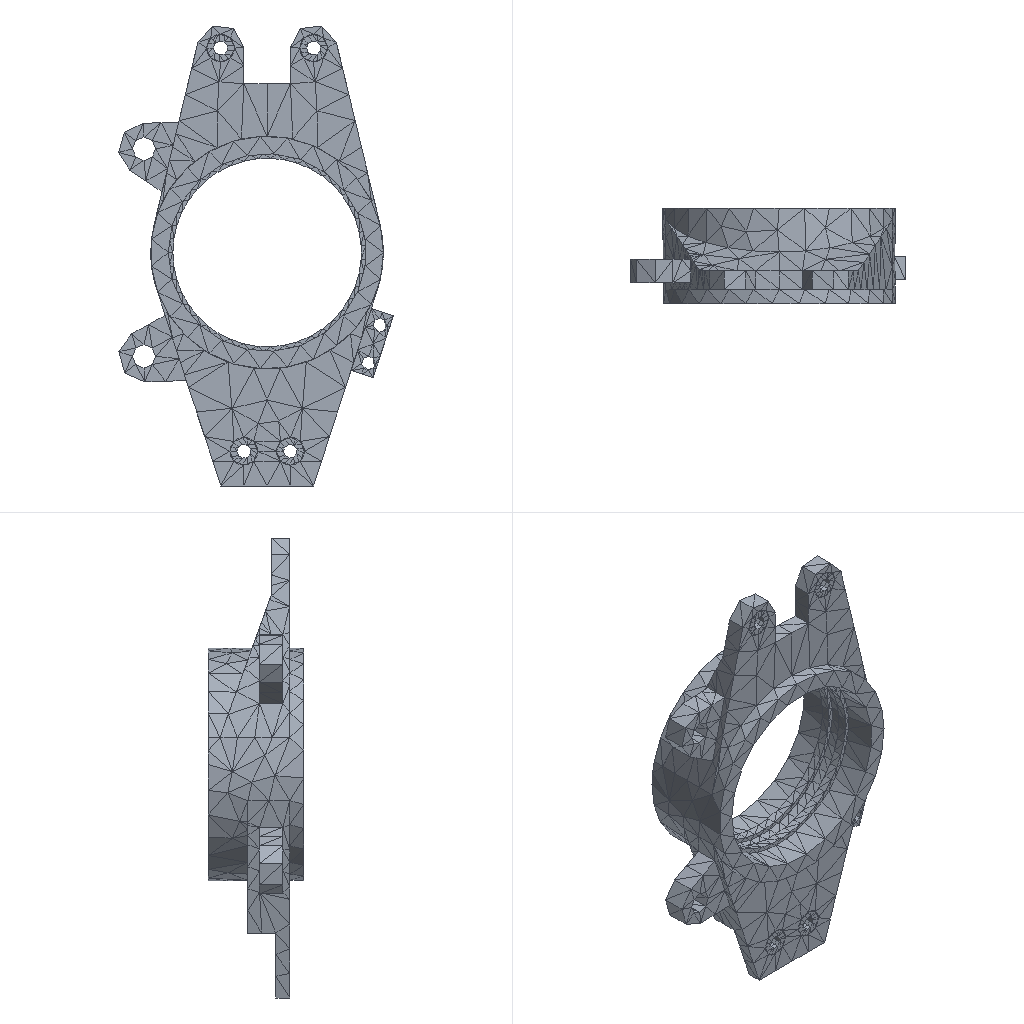Simulation study | ansys workbench
Set-up summary:
category,name,step,type,value,unit,region
solver,ansys_workbench
units,mm-N-s-tonne (MPa),,stated,"/units,MPA"
analysis,deck-1/LS1,,static
load_step,deck-1/LS1,deck-1/LS1,static,nsubst=1; time=1
analysis,deck-2/LS1,,static
load_step,deck-2/LS1,deck-2/LS1,static,nsubst=1; time=1
analysis,deck-3/LS1,,static
load_step,deck-3/LS1,deck-3/LS1,static,nsubst=1; time=1
mesh,deck-1.dat,,nodes,7389
mesh,deck-1.dat,,elements,3693
element_type,SOLID187,,,2770,,deck-1.dat
element_type,TARGE170,,,302,,deck-1.dat
element_type,CONTA174,,,302,,deck-1.dat
element_type,SOLID186,,,266,,deck-1.dat
element_type,SURF154,,,53,,deck-1.dat
mesh,deck-2.dat,,nodes,7389
mesh,deck-2.dat,,elements,3763
element_type,SOLID187,,,2770,,deck-2.dat
element_type,TARGE170,,,302,,deck-2.dat
element_type,CONTA174,,,302,,deck-2.dat
element_type,SOLID186,,,266,,deck-2.dat
element_type,SURF156,,,123,,deck-2.dat
mesh,deck-3.dat,,nodes,7390
mesh,deck-3.dat,,elements,3761
element_type,SOLID187,,,2770,,deck-3.dat
element_type,TARGE170,,,302,,deck-3.dat
element_type,CONTA174,,,302,,deck-3.dat
element_type,SOLID186,,,266,,deck-3.dat
element_type,CONTA177,,,121,,deck-3.dat
material,Aluminum 6061-T6; 6061-T651,,E,68950,tonne s^-2 mm^-1
material,Aluminum 6061-T6; 6061-T651,,nu,0.33
material,Aluminum 6061-T6; 6061-T651,,density,2.7e-09,tonne mm^-3
material,Aluminum 6061-T6; 6061-T651,,conductivity,167.2,tonne mm s^-3 C^-1
material,Aluminum 6061-T6; 6061-T651,,specific_heat,8.96e+08,mm^2 s^-2 C^-1
material,Aluminum 6061-T6; 6061-T651,,cte,7.88861e-31,C^-1
material,Aluminum 6061-T6; 6061-T651,,E,68950,tonne s^-2 mm^-1
material,Aluminum 6061-T6; 6061-T651,,nu,0.33
material,Aluminum 6061-T6; 6061-T651,,density,2.7e-09,tonne mm^-3
material,Aluminum 6061-T6; 6061-T651,,conductivity,167.2,tonne mm s^-3 C^-1
material,Aluminum 6061-T6; 6061-T651,,specific_heat,8.96e+08,mm^2 s^-2 C^-1
material,Aluminum 6061-T6; 6061-T651,,cte,7.88861e-31,C^-1
material,Aluminum 6061-T6; 6061-T651,,E,68950,tonne s^-2 mm^-1
material,Aluminum 6061-T6; 6061-T651,,nu,0.33
material,Aluminum 6061-T6; 6061-T651,,density,2.7e-09,tonne mm^-3
material,Aluminum 6061-T6; 6061-T651,,conductivity,167.2,tonne mm s^-3 C^-1
material,Aluminum 6061-T6; 6061-T651,,specific_heat,8.96e+08,mm^2 s^-2 C^-1
material,Aluminum 6061-T6; 6061-T651,,cte,7.88861e-31,C^-1
load,Define Force Using Surface Effect Elements,deck-1/LS1,surface-effect pres face 1,-3.50756e-05,,SURF154 #14
load,Define Force Using Surface Effect Elements,deck-1/LS1,surface-effect pres face 2,-0.78,,SURF154 #14
load,Define Force Using Surface Effect Elements,deck-1/LS1,surface-effect pres face 3,1.75561e-16,,SURF154 #14
load,Define Line Pressure Vector Using Surface Effect Elements,deck-2/LS1,surface-effect pres face 1,318,,SURF156 #14
load,,deck-3/LS1,moment,"288 [dir=(0, 1, 0) n=3]",,all
bc,Fixed Supports,deck-1/model,fixed,[dofs=ALL],,_FIXEDSU
bc,Fixed Supports,deck-2/model,fixed,[dofs=ALL],,_FIXEDSU
bc,Fixed Supports,deck-3/model,fixed,[dofs=ALL],,_FIXEDSU
contact,Contact Region,,bonded (always),element=CONTA174
contact,Contact Region 2,,bonded (always),element=CONTA174
contact,Contact Region 3,,bonded (always),element=CONTA174
contact,Contact Region 4,,bonded (always),element=CONTA174
contact,Contact Region,,bonded (always),element=CONTA174
contact,Contact Region 2,,bonded (always),element=CONTA174
contact,Contact Region 3,,bonded (always),element=CONTA174
contact,Contact Region 4,,bonded (always),element=CONTA174
contact,Contact Region,,bonded (always),element=CONTA174
contact,Contact Region 2,,bonded (always),element=CONTA174
contact,Contact Region 3,,bonded (always),element=CONTA174
contact,Contact Region 4,,bonded (always),element=CONTA174
contact,contact 5,,bonded (always),element=CONTA177
named_set,_FIXEDSU,,node,670
named_set,_FIXEDSU,,node,544
named_set,_FIXEDSU,,node,498
Results summary:
result,analyses[0].index,,,1
result,analyses[0].system,,,SYS
result,analyses[0].deck,,,deck-1.dat
result,analyses[0].solve_status,,,completed
result,analyses[0].analysis_type,,,static
result,analyses[0].physics,,,mechanical
result,analyses[0].unit_system,,,"NMM: mm, ton, N, s, mV, mA, degC"
result,analyses[0].n_sets,,,1
result,analyses[0].load_steps[0].set,set=1,,1
result,analyses[0].load_steps[0].time_or_freq,set=1,,1
result,analyses[0].load_steps[0].max_displacement_magnitude,set=1,,0.01102
result,analyses[0].load_steps[0].max_von_mises_nodal,set=1,,26.752
result,analyses[0].load_steps[0].reaction_force_sum_xyz[1],set=1,,0.07645
result,analyses[0].load_steps[0].reaction_force_sum_xyz[2],set=1,,1700
result,analyses[0].load_steps[0].reaction_force_sum_xyz[3],set=1,,6.14868e-11
result,analyses[1].index,,,2
result,analyses[1].system,,,SYS-1
result,analyses[1].deck,,,deck-2.dat
result,analyses[1].solve_status,,,completed
result,analyses[1].analysis_type,,,static
result,analyses[1].physics,,,mechanical
result,analyses[1].unit_system,,,"NMM: mm, ton, N, s, mV, mA, degC"
result,analyses[1].n_sets,,,1
result,analyses[1].load_steps[0].set,set=1,,1
result,analyses[1].load_steps[0].time_or_freq,set=1,,1
result,analyses[1].load_steps[0].max_displacement_magnitude,set=1,,2.114
result,analyses[1].load_steps[0].max_von_mises_nodal,set=1,,2142.6
result,analyses[1].load_steps[0].reaction_force_sum_xyz[1],set=1,,-293210
result,analyses[1].load_steps[0].reaction_force_sum_xyz[2],set=1,,-4.62397e-08
result,analyses[1].load_steps[0].reaction_force_sum_xyz[3],set=1,,-1.30146e-08
result,analyses[2].index,,,3
result,analyses[2].system,,,SYS-2
result,analyses[2].deck,,,deck-3.dat
result,analyses[2].solve_status,,,completed
result,analyses[2].analysis_type,,,static
result,analyses[2].physics,,,mechanical
result,analyses[2].unit_system,,,"NMM: mm, ton, N, s, mV, mA, degC"
result,analyses[2].n_sets,,,1
result,analyses[2].load_steps[0].set,set=1,,1
result,analyses[2].load_steps[0].time_or_freq,set=1,,1
result,analyses[2].load_steps[0].max_displacement_magnitude,set=1,,1.48821e-05
result,analyses[2].load_steps[0].max_von_mises_nodal,set=1,,0.04386
result,analyses[2].load_steps[0].reaction_force_sum_xyz[1],set=1,,-1.00805e-14
result,analyses[2].load_steps[0].reaction_force_sum_xyz[2],set=1,,2.98812e-13
result,analyses[2].load_steps[0].reaction_force_sum_xyz[3],set=1,,5.47496e-14
result,geometry_export[0][0],,,.step
result,geometry_export[0][1],,,ok
result,geometry_export[0][2],,,5